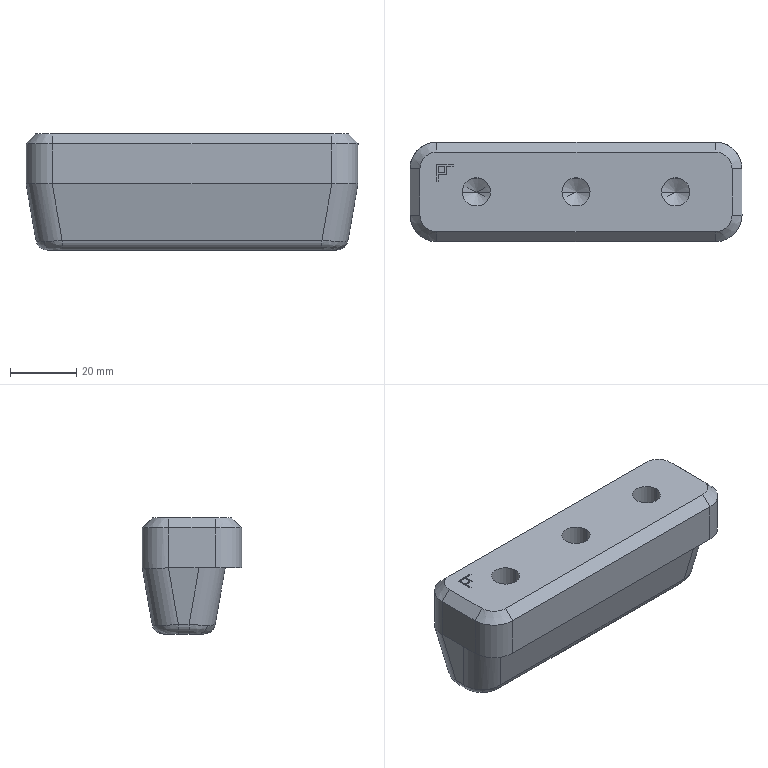Part | SolidWorks | features BaseBody 1 | 1 solid | 63 faces | box 100 x 30 x 35 mm | volume 79318 mm3 | plane 29 | cylinder 18 | cone 10 | spline 6 | commonest cylinder face diameters 16 x8 8.5 x6 7 x4